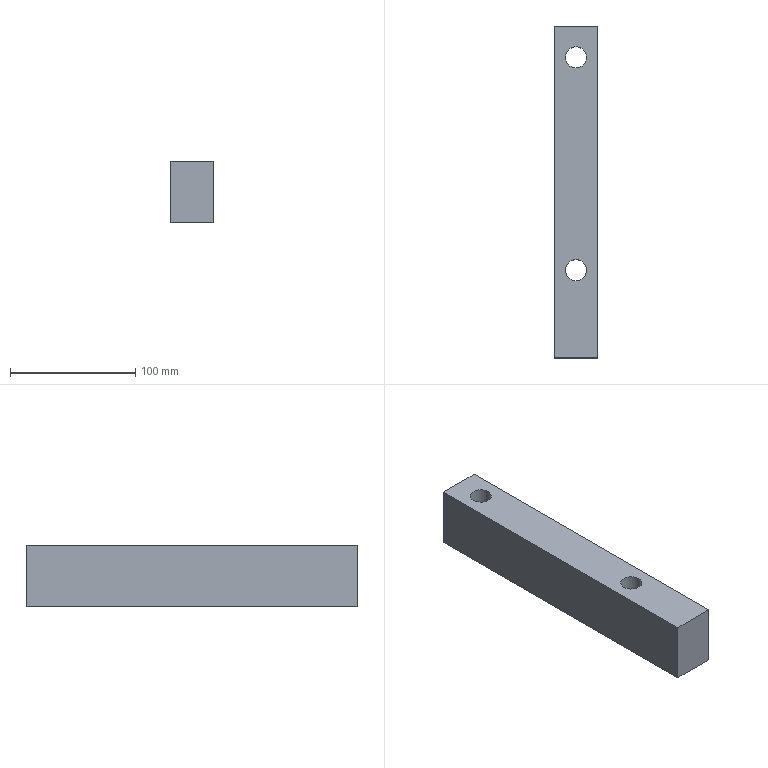Part | NX | features solid 2 | 1 solid | 8 faces | box 35 x 265 x 49 mm | volume 432231 mm3 | plane 6 | cylinder 2 | commonest cylinder face diameters 17 x2
STEP:
#1=CARTESIAN_POINT('',(668.,-105.,153.));
#2=VERTEX_POINT('',#1);
#3=CARTESIAN_POINT('',(668.,-105.,202.));
#4=VERTEX_POINT('',#3);
#5=CARTESIAN_POINT('',(668.,-105.,148.));
#6=DIRECTION('',(0.,0.,1.));
#7=VECTOR('',#6,1000.);
#8=LINE('',#5,#7);
#9=EDGE_CURVE('',#2,#4,#8,.T.);
#10=ORIENTED_EDGE('',*,*,#9,.F.);
#11=CARTESIAN_POINT('',(668.,-370.,153.));
#12=VERTEX_POINT('',#11);
#13=CARTESIAN_POINT('',(668.,0.,153.));
#14=DIRECTION('',(0.,-1.,0.));
#15=VECTOR('',#14,1000.);
#16=LINE('',#13,#15);
#17=EDGE_CURVE('',#2,#12,#16,.T.);
#18=ORIENTED_EDGE('',*,*,#17,.T.);
#19=CARTESIAN_POINT('',(668.,-370.,202.));
#20=VERTEX_POINT('',#19);
#21=CARTESIAN_POINT('',(668.,-370.,148.));
#22=DIRECTION('',(0.,0.,1.));
#23=VECTOR('',#22,1000.);
#24=LINE('',#21,#23);
#25=EDGE_CURVE('',#12,#20,#24,.T.);
#26=ORIENTED_EDGE('',*,*,#25,.T.);
#27=CARTESIAN_POINT('',(668.,0.,202.));
#28=DIRECTION('',(0.,-1.,0.));
#29=VECTOR('',#28,1000.);
#30=LINE('',#27,#29);
#31=EDGE_CURVE('',#4,#20,#30,.T.);
#32=ORIENTED_EDGE('',*,*,#31,.F.);
#33=EDGE_LOOP('',(#10,#18,#26,#32));
#34=FACE_BOUND('',#33,.T.);
#35=CARTESIAN_POINT('',(668.,0.,148.));
#36=DIRECTION('',(-1.,0.,0.));
#37=DIRECTION('',(0.,0.,1.));
#38=AXIS2_PLACEMENT_3D('',#35,#36,#37);
#39=PLANE('',#38);
#40=ADVANCED_FACE('',(#34),#39,.T.);
#41=ORIENTED_EDGE('',*,*,#25,.F.);
#42=CARTESIAN_POINT('',(703.,-370.,153.));
#43=VERTEX_POINT('',#42);
#44=CARTESIAN_POINT('',(685.5,-370.,153.));
#45=DIRECTION('',(1.,0.,0.));
#46=VECTOR('',#45,1000.);
#47=LINE('',#44,#46);
#48=EDGE_CURVE('',#12,#43,#47,.T.);
#49=ORIENTED_EDGE('',*,*,#48,.T.);
#50=CARTESIAN_POINT('',(703.,-370.,202.));
#51=VERTEX_POINT('',#50);
#52=CARTESIAN_POINT('',(703.,-370.,148.));
#53=DIRECTION('',(0.,0.,1.));
#54=VECTOR('',#53,1000.);
#55=LINE('',#52,#54);
#56=EDGE_CURVE('',#43,#51,#55,.T.);
#57=ORIENTED_EDGE('',*,*,#56,.T.);
#58=CARTESIAN_POINT('',(685.5,-370.,202.));
#59=DIRECTION('',(1.,0.,0.));
#60=VECTOR('',#59,1000.);
#61=LINE('',#58,#60);
#62=EDGE_CURVE('',#20,#51,#61,.T.);
#63=ORIENTED_EDGE('',*,*,#62,.F.);
#64=EDGE_LOOP('',(#41,#49,#57,#63));
#65=FACE_BOUND('',#64,.T.);
#66=CARTESIAN_POINT('',(685.5,-370.,148.));
#67=DIRECTION('',(0.,-1.,0.));
#68=DIRECTION('',(0.,0.,1.));
#69=AXIS2_PLACEMENT_3D('',#66,#67,#68);
#70=PLANE('',#69);
#71=ADVANCED_FACE('',(#65),#70,.T.);
#72=ORIENTED_EDGE('',*,*,#56,.F.);
#73=CARTESIAN_POINT('',(703.,-105.,153.));
#74=VERTEX_POINT('',#73);
#75=CARTESIAN_POINT('',(703.,0.,153.));
#76=DIRECTION('',(0.,1.,0.));
#77=VECTOR('',#76,1000.);
#78=LINE('',#75,#77);
#79=EDGE_CURVE('',#43,#74,#78,.T.);
#80=ORIENTED_EDGE('',*,*,#79,.T.);
#81=CARTESIAN_POINT('',(703.,-105.,202.));
#82=VERTEX_POINT('',#81);
#83=CARTESIAN_POINT('',(703.,-105.,148.));
#84=DIRECTION('',(0.,0.,1.));
#85=VECTOR('',#84,1000.);
#86=LINE('',#83,#85);
#87=EDGE_CURVE('',#74,#82,#86,.T.);
#88=ORIENTED_EDGE('',*,*,#87,.T.);
#89=CARTESIAN_POINT('',(703.,0.,202.));
#90=DIRECTION('',(0.,1.,0.));
#91=VECTOR('',#90,1000.);
#92=LINE('',#89,#91);
#93=EDGE_CURVE('',#51,#82,#92,.T.);
#94=ORIENTED_EDGE('',*,*,#93,.F.);
#95=EDGE_LOOP('',(#72,#80,#88,#94));
#96=FACE_BOUND('',#95,.T.);
#97=CARTESIAN_POINT('',(703.,0.,148.));
#98=DIRECTION('',(1.,0.,0.));
#99=DIRECTION('',(0.,0.,-1.));
#100=AXIS2_PLACEMENT_3D('',#97,#98,#99);
#101=PLANE('',#100);
#102=ADVANCED_FACE('',(#96),#101,.T.);
#103=ORIENTED_EDGE('',*,*,#87,.F.);
#104=CARTESIAN_POINT('',(685.5,-105.,153.));
#105=DIRECTION('',(-1.,0.,0.));
#106=VECTOR('',#105,1000.);
#107=LINE('',#104,#106);
#108=EDGE_CURVE('',#74,#2,#107,.T.);
#109=ORIENTED_EDGE('',*,*,#108,.T.);
#110=ORIENTED_EDGE('',*,*,#9,.T.);
#111=CARTESIAN_POINT('',(685.5,-105.,202.));
#112=DIRECTION('',(-1.,0.,0.));
#113=VECTOR('',#112,1000.);
#114=LINE('',#111,#113);
#115=EDGE_CURVE('',#82,#4,#114,.T.);
#116=ORIENTED_EDGE('',*,*,#115,.F.);
#117=EDGE_LOOP('',(#103,#109,#110,#116));
#118=FACE_BOUND('',#117,.T.);
#119=CARTESIAN_POINT('',(685.5,-105.,148.));
#120=DIRECTION('',(0.,1.,0.));
#121=DIRECTION('',(0.,0.,-1.));
#122=AXIS2_PLACEMENT_3D('',#119,#120,#121);
#123=PLANE('',#122);
#124=ADVANCED_FACE('',(#118),#123,.T.);
#125=CARTESIAN_POINT('',(694.,-130.,202.));
#126=VERTEX_POINT('',#125);
#127=CARTESIAN_POINT('',(685.5,-130.,202.));
#128=DIRECTION('',(0.,0.,1.));
#129=DIRECTION('',(1.,0.,0.));
#130=AXIS2_PLACEMENT_3D('',#127,#128,#129);
#131=CIRCLE('',#130,8.5);
#132=EDGE_CURVE('',#126,#126,#131,.T.);
#133=ORIENTED_EDGE('',*,*,#132,.F.);
#134=EDGE_LOOP('',(#133));
#135=FACE_BOUND('',#134,.T.);
#136=CARTESIAN_POINT('',(694.,-300.,202.));
#137=VERTEX_POINT('',#136);
#138=CARTESIAN_POINT('',(685.5,-300.,202.));
#139=DIRECTION('',(0.,0.,1.));
#140=DIRECTION('',(1.,0.,0.));
#141=AXIS2_PLACEMENT_3D('',#138,#139,#140);
#142=CIRCLE('',#141,8.5);
#143=EDGE_CURVE('',#137,#137,#142,.F.);
#144=ORIENTED_EDGE('',*,*,#143,.T.);
#145=EDGE_LOOP('',(#144));
#146=FACE_BOUND('',#145,.T.);
#147=ORIENTED_EDGE('',*,*,#115,.T.);
#148=ORIENTED_EDGE('',*,*,#31,.T.);
#149=ORIENTED_EDGE('',*,*,#62,.T.);
#150=ORIENTED_EDGE('',*,*,#93,.T.);
#151=EDGE_LOOP('',(#147,#148,#149,#150));
#152=FACE_BOUND('',#151,.T.);
#153=CARTESIAN_POINT('',(685.5,0.,202.));
#154=DIRECTION('',(0.,0.,1.));
#155=DIRECTION('',(1.,0.,0.));
#156=AXIS2_PLACEMENT_3D('',#153,#154,#155);
#157=PLANE('',#156);
#158=ADVANCED_FACE('',(#135,#146,#152),#157,.T.);
#159=CARTESIAN_POINT('',(677.,-130.,153.));
#160=VERTEX_POINT('',#159);
#161=CARTESIAN_POINT('',(685.5,-130.,153.));
#162=DIRECTION('',(0.,0.,-1.));
#163=DIRECTION('',(-1.,0.,0.));
#164=AXIS2_PLACEMENT_3D('',#161,#162,#163);
#165=CIRCLE('',#164,8.5);
#166=EDGE_CURVE('',#160,#160,#165,.T.);
#167=ORIENTED_EDGE('',*,*,#166,.F.);
#168=EDGE_LOOP('',(#167));
#169=FACE_BOUND('',#168,.T.);
#170=CARTESIAN_POINT('',(677.,-300.,153.));
#171=VERTEX_POINT('',#170);
#172=CARTESIAN_POINT('',(685.5,-300.,153.));
#173=DIRECTION('',(0.,0.,-1.));
#174=DIRECTION('',(-1.,0.,0.));
#175=AXIS2_PLACEMENT_3D('',#172,#173,#174);
#176=CIRCLE('',#175,8.5);
#177=EDGE_CURVE('',#171,#171,#176,.F.);
#178=ORIENTED_EDGE('',*,*,#177,.T.);
#179=EDGE_LOOP('',(#178));
#180=FACE_BOUND('',#179,.T.);
#181=ORIENTED_EDGE('',*,*,#17,.F.);
#182=ORIENTED_EDGE('',*,*,#108,.F.);
#183=ORIENTED_EDGE('',*,*,#79,.F.);
#184=ORIENTED_EDGE('',*,*,#48,.F.);
#185=EDGE_LOOP('',(#181,#182,#183,#184));
#186=FACE_BOUND('',#185,.T.);
#187=CARTESIAN_POINT('',(835.5,0.,153.));
#188=DIRECTION('',(0.,0.,-1.));
#189=DIRECTION('',(-1.,0.,0.));
#190=AXIS2_PLACEMENT_3D('',#187,#188,#189);
#191=PLANE('',#190);
#192=ADVANCED_FACE('',(#169,#180,#186),#191,.T.);
#193=ORIENTED_EDGE('',*,*,#143,.F.);
#194=EDGE_LOOP('',(#193));
#195=FACE_BOUND('',#194,.T.);
#196=ORIENTED_EDGE('',*,*,#177,.F.);
#197=EDGE_LOOP('',(#196));
#198=FACE_BOUND('',#197,.T.);
#199=CARTESIAN_POINT('',(685.5,-300.,69.));
#200=DIRECTION('',(0.,0.,1.));
#201=DIRECTION('',(1.,0.,0.));
#202=AXIS2_PLACEMENT_3D('',#199,#200,#201);
#203=CYLINDRICAL_SURFACE('',#202,8.5);
#204=ADVANCED_FACE('',(#195,#198),#203,.F.);
#205=ORIENTED_EDGE('',*,*,#132,.T.);
#206=EDGE_LOOP('',(#205));
#207=FACE_BOUND('',#206,.T.);
#208=ORIENTED_EDGE('',*,*,#166,.T.);
#209=EDGE_LOOP('',(#208));
#210=FACE_BOUND('',#209,.T.);
#211=CARTESIAN_POINT('',(685.5,-130.,69.));
#212=DIRECTION('',(0.,0.,1.));
#213=DIRECTION('',(1.,0.,0.));
#214=AXIS2_PLACEMENT_3D('',#211,#212,#213);
#215=CYLINDRICAL_SURFACE('',#214,8.5);
#216=ADVANCED_FACE('',(#207,#210),#215,.F.);
#217=CLOSED_SHELL('',(#40,#71,#102,#124,#158,#192,#204,#216));
#218=MANIFOLD_SOLID_BREP('',#217);
#219=(LENGTH_UNIT()NAMED_UNIT(*)SI_UNIT(.MILLI.,.METRE.));
#220=UNCERTAINTY_MEASURE_WITH_UNIT(LENGTH_MEASURE(0.00001),#219,'','');
#221=(NAMED_UNIT(*)PLANE_ANGLE_UNIT()SI_UNIT($,.RADIAN.));
#222=(NAMED_UNIT(*)SI_UNIT($,.STERADIAN.)SOLID_ANGLE_UNIT());
#223=(GEOMETRIC_REPRESENTATION_CONTEXT(3)GLOBAL_UNCERTAINTY_ASSIGNED_CONTEXT((#220))GLOBAL_UNIT_ASSIGNED_CONTEXT((#219,#221,#222))REPRESENTATION_CONTEXT('',''));
#224=ADVANCED_BREP_SHAPE_REPRESENTATION('',(#218),#223);